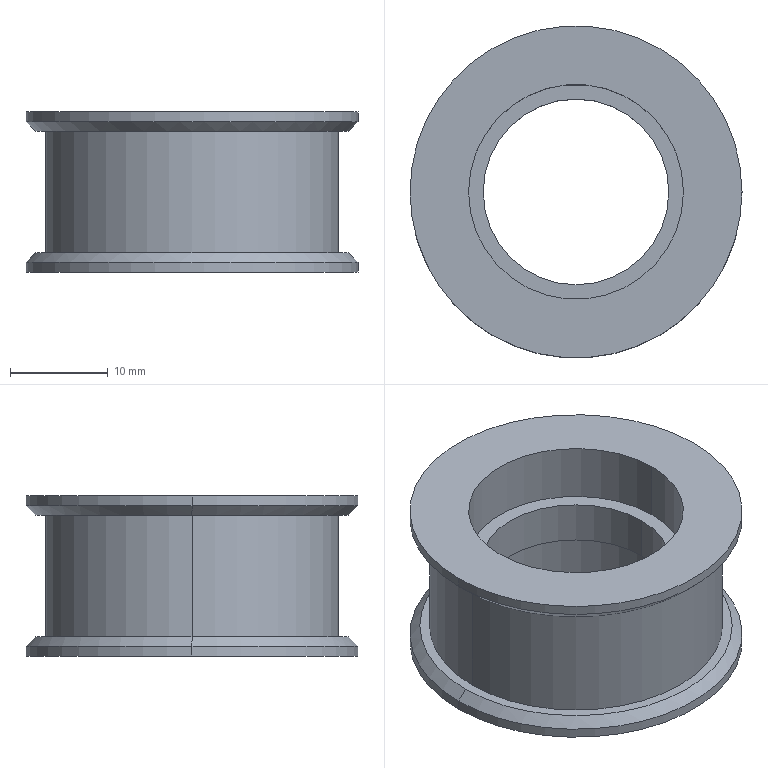Part | STEP file | PN_0033 Mount electronic clip wheel connector | 1 solid | 22 faces | box 34 x 34 x 16.4 mm | volume 6483 mm3 | cylinder 12 | plane 6 | cone 4 | commonest cylinder face diameters 22 x4 34 x4 19 x2 30 x2
STEP:
#1=CARTESIAN_POINT('',(0.,0.,0.));
#2=DIRECTION('',(0.,0.,1.));
#3=DIRECTION('',(1.,0.,0.));
#4=AXIS2_PLACEMENT_3D('',#1,#2,#3);
#5=CARTESIAN_POINT('',(16.,0.,0.));
#6=VERTEX_POINT('',#5);
#7=CARTESIAN_POINT('',(-16.,0.,0.));
#8=VERTEX_POINT('',#7);
#9=CARTESIAN_POINT('',(0.,0.,0.));
#10=DIRECTION('',(0.,0.,1.));
#11=DIRECTION('',(-1.,0.,0.));
#12=AXIS2_PLACEMENT_3D('',#9,#10,#11);
#13=CIRCLE('',#12,16.);
#14=CARTESIAN_POINT('',(0.,0.,-1.));
#15=DIRECTION('',(0.,0.,-1.));
#16=DIRECTION('',(-1.,0.,0.));
#17=AXIS2_PLACEMENT_3D('',#14,#15,#16);
#18=CONICAL_SURFACE('',#17,17.,0.7854);
#19=CARTESIAN_POINT('',(6.283,-1.));
#20=DIRECTION('',(-1.,0.));
#21=VECTOR('',#20,1.);
#22=LINE('',#19,#21);
#23=(GEOMETRIC_REPRESENTATION_CONTEXT(2)PARAMETRIC_REPRESENTATION_CONTEXT()REPRESENTATION_CONTEXT('',''));
#24=DEFINITIONAL_REPRESENTATION('',(#22),#23);
#25=PCURVE('',#18,#24);
#26=CARTESIAN_POINT('',(0.,0.,0.));
#27=DIRECTION('',(0.,0.,-1.));
#28=DIRECTION('',(-1.,0.,0.));
#29=AXIS2_PLACEMENT_3D('',#26,#27,#28);
#30=PLANE('',#29);
#31=CARTESIAN_POINT('',(16.,0.));
#32=CARTESIAN_POINT('',(16.,-27.713));
#33=CARTESIAN_POINT('',(-8.,-13.856));
#34=CARTESIAN_POINT('',(-32.,0.));
#35=CARTESIAN_POINT('',(-8.,13.856));
#36=CARTESIAN_POINT('',(16.,27.713));
#37=CARTESIAN_POINT('',(16.,0.));
#38=(BOUNDED_CURVE()B_SPLINE_CURVE(2,(#31,#32,#33,#34,#35,#36,#37),.UNSPECIFIED.,.T.,.F.)B_SPLINE_CURVE_WITH_KNOTS((1,2,2,2,2,1),(-2.094,0.,2.094,4.189,6.283,8.378),.UNSPECIFIED.)CURVE()GEOMETRIC_REPRESENTATION_ITEM()RATIONAL_B_SPLINE_CURVE((1.,0.5,1.,0.5,1.,0.5,1.))REPRESENTATION_ITEM(''));
#39=(GEOMETRIC_REPRESENTATION_CONTEXT(2)PARAMETRIC_REPRESENTATION_CONTEXT()REPRESENTATION_CONTEXT('',''));
#40=DEFINITIONAL_REPRESENTATION('',(#38),#39);
#41=PCURVE('',#30,#40);
#42=SURFACE_CURVE('',#13,(#25,#41),.PCURVE_S1.);
#43=EDGE_CURVE('',#6,#8,#42,.T.);
#44=ORIENTED_EDGE('',*,*,#43,.F.);
#45=CARTESIAN_POINT('',(17.,0.,-1.));
#46=VERTEX_POINT('',#45);
#47=CARTESIAN_POINT('',(17.,0.,-1.));
#48=DIRECTION('',(0.7071,0.,-0.7071));
#49=VECTOR('',#48,1.);
#50=LINE('',#47,#49);
#51=CARTESIAN_POINT('',(3.142,0.));
#52=DIRECTION('',(0.,1.));
#53=VECTOR('',#52,1.);
#54=LINE('',#51,#53);
#55=(GEOMETRIC_REPRESENTATION_CONTEXT(2)PARAMETRIC_REPRESENTATION_CONTEXT()REPRESENTATION_CONTEXT('',''));
#56=DEFINITIONAL_REPRESENTATION('',(#54),#55);
#57=PCURVE('',#18,#56);
#58=CARTESIAN_POINT('',(0.,0.,-1.));
#59=DIRECTION('',(0.,0.,-1.));
#60=DIRECTION('',(-1.,0.,0.));
#61=AXIS2_PLACEMENT_3D('',#58,#59,#60);
#62=CONICAL_SURFACE('',#61,17.,0.7854);
#63=CARTESIAN_POINT('',(3.142,0.));
#64=DIRECTION('',(0.,1.));
#65=VECTOR('',#64,1.);
#66=LINE('',#63,#65);
#67=(GEOMETRIC_REPRESENTATION_CONTEXT(2)PARAMETRIC_REPRESENTATION_CONTEXT()REPRESENTATION_CONTEXT('',''));
#68=DEFINITIONAL_REPRESENTATION('',(#66),#67);
#69=PCURVE('',#62,#68);
#70=SURFACE_CURVE('',#50,(#57,#69),.PCURVE_S1.);
#71=EDGE_CURVE('',#6,#46,#70,.T.);
#72=ORIENTED_EDGE('',*,*,#71,.T.);
#73=CARTESIAN_POINT('',(-17.,0.,-1.));
#74=VERTEX_POINT('',#73);
#75=CARTESIAN_POINT('',(0.,0.,-1.));
#76=DIRECTION('',(0.,0.,-1.));
#77=DIRECTION('',(-1.,0.,0.));
#78=AXIS2_PLACEMENT_3D('',#75,#76,#77);
#79=CIRCLE('',#78,17.);
#80=CARTESIAN_POINT('',(0.,0.));
#81=DIRECTION('',(1.,0.));
#82=VECTOR('',#81,1.);
#83=LINE('',#80,#82);
#84=(GEOMETRIC_REPRESENTATION_CONTEXT(2)PARAMETRIC_REPRESENTATION_CONTEXT()REPRESENTATION_CONTEXT('',''));
#85=DEFINITIONAL_REPRESENTATION('',(#83),#84);
#86=PCURVE('',#18,#85);
#87=CARTESIAN_POINT('',(0.,0.,-2.));
#88=DIRECTION('',(0.,0.,1.));
#89=DIRECTION('',(1.,0.,0.));
#90=AXIS2_PLACEMENT_3D('',#87,#88,#89);
#91=CYLINDRICAL_SURFACE('',#90,17.);
#92=CARTESIAN_POINT('',(3.142,1.));
#93=DIRECTION('',(-1.,0.));
#94=VECTOR('',#93,1.);
#95=LINE('',#92,#94);
#96=(GEOMETRIC_REPRESENTATION_CONTEXT(2)PARAMETRIC_REPRESENTATION_CONTEXT()REPRESENTATION_CONTEXT('',''));
#97=DEFINITIONAL_REPRESENTATION('',(#95),#96);
#98=PCURVE('',#91,#97);
#99=SURFACE_CURVE('',#79,(#86,#98),.PCURVE_S1.);
#100=EDGE_CURVE('',#74,#46,#99,.T.);
#101=ORIENTED_EDGE('',*,*,#100,.F.);
#102=CARTESIAN_POINT('',(-17.,0.,-1.));
#103=DIRECTION('',(-0.7071,0.,-0.7071));
#104=VECTOR('',#103,1.);
#105=LINE('',#102,#104);
#106=CARTESIAN_POINT('',(0.,0.));
#107=DIRECTION('',(0.,1.));
#108=VECTOR('',#107,1.);
#109=LINE('',#106,#108);
#110=(GEOMETRIC_REPRESENTATION_CONTEXT(2)PARAMETRIC_REPRESENTATION_CONTEXT()REPRESENTATION_CONTEXT('',''));
#111=DEFINITIONAL_REPRESENTATION('',(#109),#110);
#112=PCURVE('',#18,#111);
#113=CARTESIAN_POINT('',(6.283,0.));
#114=DIRECTION('',(0.,1.));
#115=VECTOR('',#114,1.);
#116=LINE('',#113,#115);
#117=(GEOMETRIC_REPRESENTATION_CONTEXT(2)PARAMETRIC_REPRESENTATION_CONTEXT()REPRESENTATION_CONTEXT('',''));
#118=DEFINITIONAL_REPRESENTATION('',(#116),#117);
#119=PCURVE('',#62,#118);
#120=SURFACE_CURVE('',#105,(#112,#119),.PCURVE_S1.);
#121=EDGE_CURVE('',#8,#74,#120,.T.);
#122=ORIENTED_EDGE('',*,*,#121,.F.);
#123=EDGE_LOOP('',(#44,#72,#101,#122));
#124=FACE_BOUND('',#123,.T.);
#125=ADVANCED_FACE('',(#124),#18,.T.);
#126=CARTESIAN_POINT('',(-16.,0.,12.4));
#127=VERTEX_POINT('',#126);
#128=CARTESIAN_POINT('',(16.,0.,12.4));
#129=VERTEX_POINT('',#128);
#130=CARTESIAN_POINT('',(0.,0.,12.4));
#131=DIRECTION('',(0.,0.,-1.));
#132=DIRECTION('',(1.,0.,0.));
#133=AXIS2_PLACEMENT_3D('',#130,#131,#132);
#134=CIRCLE('',#133,16.);
#135=CARTESIAN_POINT('',(0.,0.,13.4));
#136=DIRECTION('',(0.,0.,1.));
#137=DIRECTION('',(1.,0.,0.));
#138=AXIS2_PLACEMENT_3D('',#135,#136,#137);
#139=CONICAL_SURFACE('',#138,17.,0.7854);
#140=CARTESIAN_POINT('',(6.283,-1.));
#141=DIRECTION('',(-1.,0.));
#142=VECTOR('',#141,1.);
#143=LINE('',#140,#142);
#144=(GEOMETRIC_REPRESENTATION_CONTEXT(2)PARAMETRIC_REPRESENTATION_CONTEXT()REPRESENTATION_CONTEXT('',''));
#145=DEFINITIONAL_REPRESENTATION('',(#143),#144);
#146=PCURVE('',#139,#145);
#147=CARTESIAN_POINT('',(0.,0.,12.4));
#148=DIRECTION('',(0.,0.,1.));
#149=DIRECTION('',(1.,0.,0.));
#150=AXIS2_PLACEMENT_3D('',#147,#148,#149);
#151=PLANE('',#150);
#152=CARTESIAN_POINT('',(16.,0.));
#153=CARTESIAN_POINT('',(16.,-27.713));
#154=CARTESIAN_POINT('',(-8.,-13.856));
#155=CARTESIAN_POINT('',(-32.,0.));
#156=CARTESIAN_POINT('',(-8.,13.856));
#157=CARTESIAN_POINT('',(16.,27.713));
#158=CARTESIAN_POINT('',(16.,0.));
#159=(BOUNDED_CURVE()B_SPLINE_CURVE(2,(#152,#153,#154,#155,#156,#157,#158),.UNSPECIFIED.,.T.,.F.)B_SPLINE_CURVE_WITH_KNOTS((1,2,2,2,2,1),(-2.094,0.,2.094,4.189,6.283,8.378),.UNSPECIFIED.)CURVE()GEOMETRIC_REPRESENTATION_ITEM()RATIONAL_B_SPLINE_CURVE((1.,0.5,1.,0.5,1.,0.5,1.))REPRESENTATION_ITEM(''));
#160=(GEOMETRIC_REPRESENTATION_CONTEXT(2)PARAMETRIC_REPRESENTATION_CONTEXT()REPRESENTATION_CONTEXT('',''));
#161=DEFINITIONAL_REPRESENTATION('',(#159),#160);
#162=PCURVE('',#151,#161);
#163=SURFACE_CURVE('',#134,(#146,#162),.PCURVE_S1.);
#164=EDGE_CURVE('',#127,#129,#163,.T.);
#165=ORIENTED_EDGE('',*,*,#164,.F.);
#166=CARTESIAN_POINT('',(-17.,0.,13.4));
#167=VERTEX_POINT('',#166);
#168=CARTESIAN_POINT('',(-17.,0.,13.4));
#169=DIRECTION('',(-0.7071,0.,0.7071));
#170=VECTOR('',#169,1.);
#171=LINE('',#168,#170);
#172=CARTESIAN_POINT('',(3.142,0.));
#173=DIRECTION('',(0.,1.));
#174=VECTOR('',#173,1.);
#175=LINE('',#172,#174);
#176=(GEOMETRIC_REPRESENTATION_CONTEXT(2)PARAMETRIC_REPRESENTATION_CONTEXT()REPRESENTATION_CONTEXT('',''));
#177=DEFINITIONAL_REPRESENTATION('',(#175),#176);
#178=PCURVE('',#139,#177);
#179=CARTESIAN_POINT('',(0.,0.,13.4));
#180=DIRECTION('',(0.,0.,1.));
#181=DIRECTION('',(1.,0.,0.));
#182=AXIS2_PLACEMENT_3D('',#179,#180,#181);
#183=CONICAL_SURFACE('',#182,17.,0.7854);
#184=CARTESIAN_POINT('',(3.142,0.));
#185=DIRECTION('',(0.,1.));
#186=VECTOR('',#185,1.);
#187=LINE('',#184,#186);
#188=(GEOMETRIC_REPRESENTATION_CONTEXT(2)PARAMETRIC_REPRESENTATION_CONTEXT()REPRESENTATION_CONTEXT('',''));
#189=DEFINITIONAL_REPRESENTATION('',(#187),#188);
#190=PCURVE('',#183,#189);
#191=SURFACE_CURVE('',#171,(#178,#190),.PCURVE_S1.);
#192=EDGE_CURVE('',#127,#167,#191,.T.);
#193=ORIENTED_EDGE('',*,*,#192,.T.);
#194=CARTESIAN_POINT('',(17.,0.,13.4));
#195=VERTEX_POINT('',#194);
#196=CARTESIAN_POINT('',(0.,0.,13.4));
#197=DIRECTION('',(0.,0.,1.));
#198=DIRECTION('',(1.,0.,0.));
#199=AXIS2_PLACEMENT_3D('',#196,#197,#198);
#200=CIRCLE('',#199,17.);
#201=CARTESIAN_POINT('',(0.,0.));
#202=DIRECTION('',(1.,0.));
#203=VECTOR('',#202,1.);
#204=LINE('',#201,#203);
#205=(GEOMETRIC_REPRESENTATION_CONTEXT(2)PARAMETRIC_REPRESENTATION_CONTEXT()REPRESENTATION_CONTEXT('',''));
#206=DEFINITIONAL_REPRESENTATION('',(#204),#205);
#207=PCURVE('',#139,#206);
#208=CARTESIAN_POINT('',(0.,0.,14.4));
#209=DIRECTION('',(0.,0.,-1.));
#210=DIRECTION('',(-1.,0.,0.));
#211=AXIS2_PLACEMENT_3D('',#208,#209,#210);
#212=CYLINDRICAL_SURFACE('',#211,17.);
#213=CARTESIAN_POINT('',(3.142,1.));
#214=DIRECTION('',(-1.,0.));
#215=VECTOR('',#214,1.);
#216=LINE('',#213,#215);
#217=(GEOMETRIC_REPRESENTATION_CONTEXT(2)PARAMETRIC_REPRESENTATION_CONTEXT()REPRESENTATION_CONTEXT('',''));
#218=DEFINITIONAL_REPRESENTATION('',(#216),#217);
#219=PCURVE('',#212,#218);
#220=SURFACE_CURVE('',#200,(#207,#219),.PCURVE_S1.);
#221=EDGE_CURVE('',#195,#167,#220,.T.);
#222=ORIENTED_EDGE('',*,*,#221,.F.);
#223=CARTESIAN_POINT('',(17.,0.,13.4));
#224=DIRECTION('',(0.7071,0.,0.7071));
#225=VECTOR('',#224,1.);
#226=LINE('',#223,#225);
#227=CARTESIAN_POINT('',(0.,0.));
#228=DIRECTION('',(0.,1.));
#229=VECTOR('',#228,1.);
#230=LINE('',#227,#229);
#231=(GEOMETRIC_REPRESENTATION_CONTEXT(2)PARAMETRIC_REPRESENTATION_CONTEXT()REPRESENTATION_CONTEXT('',''));
#232=DEFINITIONAL_REPRESENTATION('',(#230),#231);
#233=PCURVE('',#139,#232);
#234=CARTESIAN_POINT('',(6.283,0.));
#235=DIRECTION('',(0.,1.));
#236=VECTOR('',#235,1.);
#237=LINE('',#234,#236);
#238=(GEOMETRIC_REPRESENTATION_CONTEXT(2)PARAMETRIC_REPRESENTATION_CONTEXT()REPRESENTATION_CONTEXT('',''));
#239=DEFINITIONAL_REPRESENTATION('',(#237),#238);
#240=PCURVE('',#183,#239);
#241=SURFACE_CURVE('',#226,(#233,#240),.PCURVE_S1.);
#242=EDGE_CURVE('',#129,#195,#241,.T.);
#243=ORIENTED_EDGE('',*,*,#242,.F.);
#244=EDGE_LOOP('',(#165,#193,#222,#243));
#245=FACE_BOUND('',#244,.T.);
#246=ADVANCED_FACE('',(#245),#139,.T.);
#247=CARTESIAN_POINT('',(-11.,0.,4.));
#248=VERTEX_POINT('',#247);
#249=CARTESIAN_POINT('',(-11.,0.,-2.));
#250=VERTEX_POINT('',#249);
#251=CARTESIAN_POINT('',(-11.,0.,4.));
#252=DIRECTION('',(0.,0.,-1.));
#253=VECTOR('',#252,1.);
#254=LINE('',#251,#253);
#255=CARTESIAN_POINT('',(0.,0.,4.));
#256=DIRECTION('',(0.,0.,-1.));
#257=DIRECTION('',(-1.,0.,0.));
#258=AXIS2_PLACEMENT_3D('',#255,#256,#257);
#259=CYLINDRICAL_SURFACE('',#258,11.);
#260=CARTESIAN_POINT('',(6.283,0.));
#261=DIRECTION('',(0.,1.));
#262=VECTOR('',#261,1.);
#263=LINE('',#260,#262);
#264=(GEOMETRIC_REPRESENTATION_CONTEXT(2)PARAMETRIC_REPRESENTATION_CONTEXT()REPRESENTATION_CONTEXT('',''));
#265=DEFINITIONAL_REPRESENTATION('',(#263),#264);
#266=PCURVE('',#259,#265);
#267=CARTESIAN_POINT('',(0.,0.,4.));
#268=DIRECTION('',(0.,0.,-1.));
#269=DIRECTION('',(-1.,0.,0.));
#270=AXIS2_PLACEMENT_3D('',#267,#268,#269);
#271=CYLINDRICAL_SURFACE('',#270,11.);
#272=CARTESIAN_POINT('',(0.,0.));
#273=DIRECTION('',(0.,1.));
#274=VECTOR('',#273,1.);
#275=LINE('',#272,#274);
#276=(GEOMETRIC_REPRESENTATION_CONTEXT(2)PARAMETRIC_REPRESENTATION_CONTEXT()REPRESENTATION_CONTEXT('',''));
#277=DEFINITIONAL_REPRESENTATION('',(#275),#276);
#278=PCURVE('',#271,#277);
#279=SURFACE_CURVE('',#254,(#266,#278),.PCURVE_S1.);
#280=EDGE_CURVE('',#248,#250,#279,.T.);
#281=ORIENTED_EDGE('',*,*,#280,.T.);
#282=CARTESIAN_POINT('',(11.,0.,-2.));
#283=VERTEX_POINT('',#282);
#284=CARTESIAN_POINT('',(0.,0.,-2.));
#285=DIRECTION('',(0.,0.,-1.));
#286=DIRECTION('',(-1.,0.,0.));
#287=AXIS2_PLACEMENT_3D('',#284,#285,#286);
#288=CIRCLE('',#287,11.);
#289=CARTESIAN_POINT('',(0.,6.));
#290=DIRECTION('',(1.,0.));
#291=VECTOR('',#290,1.);
#292=LINE('',#289,#291);
#293=(GEOMETRIC_REPRESENTATION_CONTEXT(2)PARAMETRIC_REPRESENTATION_CONTEXT()REPRESENTATION_CONTEXT('',''));
#294=DEFINITIONAL_REPRESENTATION('',(#292),#293);
#295=PCURVE('',#259,#294);
#296=CARTESIAN_POINT('',(0.,0.,-2.));
#297=DIRECTION('',(0.,0.,-1.));
#298=DIRECTION('',(-1.,0.,0.));
#299=AXIS2_PLACEMENT_3D('',#296,#297,#298);
#300=PLANE('',#299);
#301=CARTESIAN_POINT('',(0.,0.));
#302=DIRECTION('',(1.,0.));
#303=AXIS2_PLACEMENT_2D('',#301,#302);
#304=CIRCLE('',#303,11.);
#305=(GEOMETRIC_REPRESENTATION_CONTEXT(2)PARAMETRIC_REPRESENTATION_CONTEXT()REPRESENTATION_CONTEXT('',''));
#306=DEFINITIONAL_REPRESENTATION('',(#304),#305);
#307=PCURVE('',#300,#306);
#308=SURFACE_CURVE('',#288,(#295,#307),.PCURVE_S1.);
#309=EDGE_CURVE('',#283,#250,#308,.T.);
#310=ORIENTED_EDGE('',*,*,#309,.F.);
#311=CARTESIAN_POINT('',(11.,0.,4.));
#312=VERTEX_POINT('',#311);
#313=CARTESIAN_POINT('',(11.,0.,4.));
#314=DIRECTION('',(0.,0.,-1.));
#315=VECTOR('',#314,1.);
#316=LINE('',#313,#315);
#317=CARTESIAN_POINT('',(3.142,0.));
#318=DIRECTION('',(0.,1.));
#319=VECTOR('',#318,1.);
#320=LINE('',#317,#319);
#321=(GEOMETRIC_REPRESENTATION_CONTEXT(2)PARAMETRIC_REPRESENTATION_CONTEXT()REPRESENTATION_CONTEXT('',''));
#322=DEFINITIONAL_REPRESENTATION('',(#320),#321);
#323=PCURVE('',#259,#322);
#324=CARTESIAN_POINT('',(3.142,0.));
#325=DIRECTION('',(0.,1.));
#326=VECTOR('',#325,1.);
#327=LINE('',#324,#326);
#328=(GEOMETRIC_REPRESENTATION_CONTEXT(2)PARAMETRIC_REPRESENTATION_CONTEXT()REPRESENTATION_CONTEXT('',''));
#329=DEFINITIONAL_REPRESENTATION('',(#327),#328);
#330=PCURVE('',#271,#329);
#331=SURFACE_CURVE('',#316,(#323,#330),.PCURVE_S1.);
#332=EDGE_CURVE('',#312,#283,#331,.T.);
#333=ORIENTED_EDGE('',*,*,#332,.F.);
#334=CARTESIAN_POINT('',(0.,0.,4.));
#335=DIRECTION('',(0.,0.,-1.));
#336=DIRECTION('',(-1.,0.,0.));
#337=AXIS2_PLACEMENT_3D('',#334,#335,#336);
#338=CIRCLE('',#337,11.);
#339=CARTESIAN_POINT('',(0.,0.));
#340=DIRECTION('',(1.,0.));
#341=VECTOR('',#340,1.);
#342=LINE('',#339,#341);
#343=(GEOMETRIC_REPRESENTATION_CONTEXT(2)PARAMETRIC_REPRESENTATION_CONTEXT()REPRESENTATION_CONTEXT('',''));
#344=DEFINITIONAL_REPRESENTATION('',(#342),#343);
#345=PCURVE('',#259,#344);
#346=CARTESIAN_POINT('',(0.,0.,4.));
#347=DIRECTION('',(0.,0.,-1.));
#348=DIRECTION('',(-1.,0.,0.));
#349=AXIS2_PLACEMENT_3D('',#346,#347,#348);
#350=PLANE('',#349);
#351=CARTESIAN_POINT('',(0.,0.));
#352=DIRECTION('',(1.,0.));
#353=AXIS2_PLACEMENT_2D('',#351,#352);
#354=CIRCLE('',#353,11.);
#355=(GEOMETRIC_REPRESENTATION_CONTEXT(2)PARAMETRIC_REPRESENTATION_CONTEXT()REPRESENTATION_CONTEXT('',''));
#356=DEFINITIONAL_REPRESENTATION('',(#354),#355);
#357=PCURVE('',#350,#356);
#358=SURFACE_CURVE('',#338,(#345,#357),.PCURVE_S1.);
#359=EDGE_CURVE('',#312,#248,#358,.T.);
#360=ORIENTED_EDGE('',*,*,#359,.T.);
#361=EDGE_LOOP('',(#281,#310,#333,#360));
#362=FACE_BOUND('',#361,.F.);
#363=ADVANCED_FACE('',(#362),#259,.F.);
#364=CARTESIAN_POINT('',(11.,0.,8.4));
#365=VERTEX_POINT('',#364);
#366=CARTESIAN_POINT('',(11.,0.,14.4));
#367=VERTEX_POINT('',#366);
#368=CARTESIAN_POINT('',(11.,0.,8.4));
#369=DIRECTION('',(0.,0.,1.));
#370=VECTOR('',#369,1.);
#371=LINE('',#368,#370);
#372=CARTESIAN_POINT('',(0.,0.,8.4));
#373=DIRECTION('',(0.,0.,1.));
#374=DIRECTION('',(1.,0.,0.));
#375=AXIS2_PLACEMENT_3D('',#372,#373,#374);
#376=CYLINDRICAL_SURFACE('',#375,11.);
#377=CARTESIAN_POINT('',(6.283,0.));
#378=DIRECTION('',(0.,1.));
#379=VECTOR('',#378,1.);
#380=LINE('',#377,#379);
#381=(GEOMETRIC_REPRESENTATION_CONTEXT(2)PARAMETRIC_REPRESENTATION_CONTEXT()REPRESENTATION_CONTEXT('',''));
#382=DEFINITIONAL_REPRESENTATION('',(#380),#381);
#383=PCURVE('',#376,#382);
#384=CARTESIAN_POINT('',(0.,0.,8.4));
#385=DIRECTION('',(0.,0.,1.));
#386=DIRECTION('',(1.,0.,0.));
#387=AXIS2_PLACEMENT_3D('',#384,#385,#386);
#388=CYLINDRICAL_SURFACE('',#387,11.);
#389=CARTESIAN_POINT('',(0.,0.));
#390=DIRECTION('',(0.,1.));
#391=VECTOR('',#390,1.);
#392=LINE('',#389,#391);
#393=(GEOMETRIC_REPRESENTATION_CONTEXT(2)PARAMETRIC_REPRESENTATION_CONTEXT()REPRESENTATION_CONTEXT('',''));
#394=DEFINITIONAL_REPRESENTATION('',(#392),#393);
#395=PCURVE('',#388,#394);
#396=SURFACE_CURVE('',#371,(#383,#395),.PCURVE_S1.);
#397=EDGE_CURVE('',#365,#367,#396,.T.);
#398=ORIENTED_EDGE('',*,*,#397,.T.);
#399=CARTESIAN_POINT('',(-11.,0.,14.4));
#400=VERTEX_POINT('',#399);
#401=CARTESIAN_POINT('',(0.,0.,14.4));
#402=DIRECTION('',(0.,0.,1.));
#403=DIRECTION('',(1.,0.,0.));
#404=AXIS2_PLACEMENT_3D('',#401,#402,#403);
#405=CIRCLE('',#404,11.);
#406=CARTESIAN_POINT('',(0.,6.));
#407=DIRECTION('',(1.,0.));
#408=VECTOR('',#407,1.);
#409=LINE('',#406,#408);
#410=(GEOMETRIC_REPRESENTATION_CONTEXT(2)PARAMETRIC_REPRESENTATION_CONTEXT()REPRESENTATION_CONTEXT('',''));
#411=DEFINITIONAL_REPRESENTATION('',(#409),#410);
#412=PCURVE('',#376,#411);
#413=CARTESIAN_POINT('',(0.,0.,14.4));
#414=DIRECTION('',(0.,0.,1.));
#415=DIRECTION('',(1.,0.,0.));
#416=AXIS2_PLACEMENT_3D('',#413,#414,#415);
#417=PLANE('',#416);
#418=CARTESIAN_POINT('',(0.,0.));
#419=DIRECTION('',(1.,0.));
#420=AXIS2_PLACEMENT_2D('',#418,#419);
#421=CIRCLE('',#420,11.);
#422=(GEOMETRIC_REPRESENTATION_CONTEXT(2)PARAMETRIC_REPRESENTATION_CONTEXT()REPRESENTATION_CONTEXT('',''));
#423=DEFINITIONAL_REPRESENTATION('',(#421),#422);
#424=PCURVE('',#417,#423);
#425=SURFACE_CURVE('',#405,(#412,#424),.PCURVE_S1.);
#426=EDGE_CURVE('',#400,#367,#425,.T.);
#427=ORIENTED_EDGE('',*,*,#426,.F.);
#428=CARTESIAN_POINT('',(-11.,0.,8.4));
#429=VERTEX_POINT('',#428);
#430=CARTESIAN_POINT('',(-11.,0.,8.4));
#431=DIRECTION('',(0.,0.,1.));
#432=VECTOR('',#431,1.);
#433=LINE('',#430,#432);
#434=CARTESIAN_POINT('',(3.142,0.));
#435=DIRECTION('',(0.,1.));
#436=VECTOR('',#435,1.);
#437=LINE('',#434,#436);
#438=(GEOMETRIC_REPRESENTATION_CONTEXT(2)PARAMETRIC_REPRESENTATION_CONTEXT()REPRESENTATION_CONTEXT('',''));
#439=DEFINITIONAL_REPRESENTATION('',(#437),#438);
#440=PCURVE('',#376,#439);
#441=CARTESIAN_POINT('',(3.142,0.));
#442=DIRECTION('',(0.,1.));
#443=VECTOR('',#442,1.);
#444=LINE('',#441,#443);
#445=(GEOMETRIC_REPRESENTATION_CONTEXT(2)PARAMETRIC_REPRESENTATION_CONTEXT()REPRESENTATION_CONTEXT('',''));
#446=DEFINITIONAL_REPRESENTATION('',(#444),#445);
#447=PCURVE('',#388,#446);
#448=SURFACE_CURVE('',#433,(#440,#447),.PCURVE_S1.);
#449=EDGE_CURVE('',#429,#400,#448,.T.);
#450=ORIENTED_EDGE('',*,*,#449,.F.);
#451=CARTESIAN_POINT('',(0.,0.,8.4));
#452=DIRECTION('',(0.,0.,1.));
#453=DIRECTION('',(1.,0.,0.));
#454=AXIS2_PLACEMENT_3D('',#451,#452,#453);
#455=CIRCLE('',#454,11.);
#456=CARTESIAN_POINT('',(0.,0.));
#457=DIRECTION('',(1.,0.));
#458=VECTOR('',#457,1.);
#459=LINE('',#456,#458);
#460=(GEOMETRIC_REPRESENTATION_CONTEXT(2)PARAMETRIC_REPRESENTATION_CONTEXT()REPRESENTATION_CONTEXT('',''));
#461=DEFINITIONAL_REPRESENTATION('',(#459),#460);
#462=PCURVE('',#376,#461);
#463=CARTESIAN_POINT('',(0.,0.,8.4));
#464=DIRECTION('',(0.,0.,1.));
#465=DIRECTION('',(1.,0.,0.));
#466=AXIS2_PLACEMENT_3D('',#463,#464,#465);
#467=PLANE('',#466);
#468=CARTESIAN_POINT('',(0.,0.));
#469=DIRECTION('',(1.,0.));
#470=AXIS2_PLACEMENT_2D('',#468,#469);
#471=CIRCLE('',#470,11.);
#472=(GEOMETRIC_REPRESENTATION_CONTEXT(2)PARAMETRIC_REPRESENTATION_CONTEXT()REPRESENTATION_CONTEXT('',''));
#473=DEFINITIONAL_REPRESENTATION('',(#471),#472);
#474=PCURVE('',#467,#473);
#475=SURFACE_CURVE('',#455,(#462,#474),.PCURVE_S1.);
#476=EDGE_CURVE('',#429,#365,#475,.T.);
#477=ORIENTED_EDGE('',*,*,#476,.T.);
#478=EDGE_LOOP('',(#398,#427,#450,#477));
#479=FACE_BOUND('',#478,.F.);
#480=ADVANCED_FACE('',(#479),#376,.F.);
#481=CARTESIAN_POINT('',(-17.,0.,-2.));
#482=VERTEX_POINT('',#481);
#483=CARTESIAN_POINT('',(17.,0.,-2.));
#484=VERTEX_POINT('',#483);
#485=CARTESIAN_POINT('',(0.,0.,-2.));
#486=DIRECTION('',(0.,0.,-1.));
#487=DIRECTION('',(-1.,0.,0.));
#488=AXIS2_PLACEMENT_3D('',#485,#486,#487);
#489=CIRCLE('',#488,17.);
#490=CARTESIAN_POINT('',(3.142,0.));
#491=DIRECTION('',(-1.,0.));
#492=VECTOR('',#491,1.);
#493=LINE('',#490,#492);
#494=(GEOMETRIC_REPRESENTATION_CONTEXT(2)PARAMETRIC_REPRESENTATION_CONTEXT()REPRESENTATION_CONTEXT('',''));
#495=DEFINITIONAL_REPRESENTATION('',(#493),#494);
#496=PCURVE('',#91,#495);
#497=CARTESIAN_POINT('',(0.,0.));
#498=DIRECTION('',(1.,0.));
#499=AXIS2_PLACEMENT_2D('',#497,#498);
#500=CIRCLE('',#499,17.);
#501=(GEOMETRIC_REPRESENTATION_CONTEXT(2)PARAMETRIC_REPRESENTATION_CONTEXT()REPRESENTATION_CONTEXT('',''));
#502=DEFINITIONAL_REPRESENTATION('',(#500),#501);
#503=PCURVE('',#300,#502);
#504=SURFACE_CURVE('',#489,(#496,#503),.PCURVE_S1.);
#505=EDGE_CURVE('',#482,#484,#504,.T.);
#506=ORIENTED_EDGE('',*,*,#505,.F.);
#507=CARTESIAN_POINT('',(-17.,0.,-2.));
#508=DIRECTION('',(0.,0.,1.));
#509=VECTOR('',#508,1.);
#510=LINE('',#507,#509);
#511=CARTESIAN_POINT('',(3.142,0.));
#512=DIRECTION('',(0.,1.));
#513=VECTOR('',#512,1.);
#514=LINE('',#511,#513);
#515=(GEOMETRIC_REPRESENTATION_CONTEXT(2)PARAMETRIC_REPRESENTATION_CONTEXT()REPRESENTATION_CONTEXT('',''));
#516=DEFINITIONAL_REPRESENTATION('',(#514),#515);
#517=PCURVE('',#91,#516);
#518=CARTESIAN_POINT('',(0.,0.,-2.));
#519=DIRECTION('',(0.,0.,1.));
#520=DIRECTION('',(1.,0.,0.));
#521=AXIS2_PLACEMENT_3D('',#518,#519,#520);
#522=CYLINDRICAL_SURFACE('',#521,17.);
#523=CARTESIAN_POINT('',(3.142,0.));
#524=DIRECTION('',(0.,1.));
#525=VECTOR('',#524,1.);
#526=LINE('',#523,#525);
#527=(GEOMETRIC_REPRESENTATION_CONTEXT(2)PARAMETRIC_REPRESENTATION_CONTEXT()REPRESENTATION_CONTEXT('',''));
#528=DEFINITIONAL_REPRESENTATION('',(#526),#527);
#529=PCURVE('',#522,#528);
#530=SURFACE_CURVE('',#510,(#517,#529),.PCURVE_S1.);
#531=EDGE_CURVE('',#482,#74,#530,.T.);
#532=ORIENTED_EDGE('',*,*,#531,.T.);
#533=ORIENTED_EDGE('',*,*,#100,.T.);
#534=CARTESIAN_POINT('',(17.,0.,-2.));
#535=DIRECTION('',(0.,0.,1.));
#536=VECTOR('',#535,1.);
#537=LINE('',#534,#536);
#538=CARTESIAN_POINT('',(0.,0.));
#539=DIRECTION('',(0.,1.));
#540=VECTOR('',#539,1.);
#541=LINE('',#538,#540);
#542=(GEOMETRIC_REPRESENTATION_CONTEXT(2)PARAMETRIC_REPRESENTATION_CONTEXT()REPRESENTATION_CONTEXT('',''));
#543=DEFINITIONAL_REPRESENTATION('',(#541),#542);
#544=PCURVE('',#91,#543);
#545=CARTESIAN_POINT('',(6.283,0.));
#546=DIRECTION('',(0.,1.));
#547=VECTOR('',#546,1.);
#548=LINE('',#545,#547);
#549=(GEOMETRIC_REPRESENTATION_CONTEXT(2)PARAMETRIC_REPRESENTATION_CONTEXT()REPRESENTATION_CONTEXT('',''));
#550=DEFINITIONAL_REPRESENTATION('',(#548),#549);
#551=PCURVE('',#522,#550);
#552=SURFACE_CURVE('',#537,(#544,#551),.PCURVE_S1.);
#553=EDGE_CURVE('',#484,#46,#552,.T.);
#554=ORIENTED_EDGE('',*,*,#553,.F.);
#555=EDGE_LOOP('',(#506,#532,#533,#554));
#556=FACE_BOUND('',#555,.T.);
#557=ADVANCED_FACE('',(#556),#91,.T.);
#558=CARTESIAN_POINT('',(17.,0.,14.4));
#559=VERTEX_POINT('',#558);
#560=CARTESIAN_POINT('',(-17.,0.,14.4));
#561=VERTEX_POINT('',#560);
#562=CARTESIAN_POINT('',(0.,0.,14.4));
#563=DIRECTION('',(0.,0.,1.));
#564=DIRECTION('',(1.,0.,0.));
#565=AXIS2_PLACEMENT_3D('',#562,#563,#564);
#566=CIRCLE('',#565,17.);
#567=CARTESIAN_POINT('',(3.142,0.));
#568=DIRECTION('',(-1.,0.));
#569=VECTOR('',#568,1.);
#570=LINE('',#567,#569);
#571=(GEOMETRIC_REPRESENTATION_CONTEXT(2)PARAMETRIC_REPRESENTATION_CONTEXT()REPRESENTATION_CONTEXT('',''));
#572=DEFINITIONAL_REPRESENTATION('',(#570),#571);
#573=PCURVE('',#212,#572);
#574=CARTESIAN_POINT('',(0.,0.));
#575=DIRECTION('',(1.,0.));
#576=AXIS2_PLACEMENT_2D('',#574,#575);
#577=CIRCLE('',#576,17.);
#578=(GEOMETRIC_REPRESENTATION_CONTEXT(2)PARAMETRIC_REPRESENTATION_CONTEXT()REPRESENTATION_CONTEXT('',''));
#579=DEFINITIONAL_REPRESENTATION('',(#577),#578);
#580=PCURVE('',#417,#579);
#581=SURFACE_CURVE('',#566,(#573,#580),.PCURVE_S1.);
#582=EDGE_CURVE('',#559,#561,#581,.T.);
#583=ORIENTED_EDGE('',*,*,#582,.F.);
#584=CARTESIAN_POINT('',(17.,0.,14.4));
#585=DIRECTION('',(0.,0.,-1.));
#586=VECTOR('',#585,1.);
#587=LINE('',#584,#586);
#588=CARTESIAN_POINT('',(3.142,0.));
#589=DIRECTION('',(0.,1.));
#590=VECTOR('',#589,1.);
#591=LINE('',#588,#590);
#592=(GEOMETRIC_REPRESENTATION_CONTEXT(2)PARAMETRIC_REPRESENTATION_CONTEXT()REPRESENTATION_CONTEXT('',''));
#593=DEFINITIONAL_REPRESENTATION('',(#591),#592);
#594=PCURVE('',#212,#593);
#595=CARTESIAN_POINT('',(0.,0.,14.4));
#596=DIRECTION('',(0.,0.,-1.));
#597=DIRECTION('',(-1.,0.,0.));
#598=AXIS2_PLACEMENT_3D('',#595,#596,#597);
#599=CYLINDRICAL_SURFACE('',#598,17.);
#600=CARTESIAN_POINT('',(3.142,0.));
#601=DIRECTION('',(0.,1.));
#602=VECTOR('',#601,1.);
#603=LINE('',#600,#602);
#604=(GEOMETRIC_REPRESENTATION_CONTEXT(2)PARAMETRIC_REPRESENTATION_CONTEXT()REPRESENTATION_CONTEXT('',''));
#605=DEFINITIONAL_REPRESENTATION('',(#603),#604);
#606=PCURVE('',#599,#605);
#607=SURFACE_CURVE('',#587,(#594,#606),.PCURVE_S1.);
#608=EDGE_CURVE('',#559,#195,#607,.T.);
#609=ORIENTED_EDGE('',*,*,#608,.T.);
#610=ORIENTED_EDGE('',*,*,#221,.T.);
#611=CARTESIAN_POINT('',(-17.,0.,14.4));
#612=DIRECTION('',(0.,0.,-1.));
#613=VECTOR('',#612,1.);
#614=LINE('',#611,#613);
#615=CARTESIAN_POINT('',(0.,0.));
#616=DIRECTION('',(0.,1.));
#617=VECTOR('',#616,1.);
#618=LINE('',#615,#617);
#619=(GEOMETRIC_REPRESENTATION_CONTEXT(2)PARAMETRIC_REPRESENTATION_CONTEXT()REPRESENTATION_CONTEXT('',''));
#620=DEFINITIONAL_REPRESENTATION('',(#618),#619);
#621=PCURVE('',#212,#620);
#622=CARTESIAN_POINT('',(6.283,0.));
#623=DIRECTION('',(0.,1.));
#624=VECTOR('',#623,1.);
#625=LINE('',#622,#624);
#626=(GEOMETRIC_REPRESENTATION_CONTEXT(2)PARAMETRIC_REPRESENTATION_CONTEXT()REPRESENTATION_CONTEXT('',''));
#627=DEFINITIONAL_REPRESENTATION('',(#625),#626);
#628=PCURVE('',#599,#627);
#629=SURFACE_CURVE('',#614,(#621,#628),.PCURVE_S1.);
#630=EDGE_CURVE('',#561,#167,#629,.T.);
#631=ORIENTED_EDGE('',*,*,#630,.F.);
#632=EDGE_LOOP('',(#583,#609,#610,#631));
#633=FACE_BOUND('',#632,.T.);
#634=ADVANCED_FACE('',(#633),#212,.T.);
#635=CARTESIAN_POINT('',(15.,0.,12.4));
#636=VERTEX_POINT('',#635);
#637=CARTESIAN_POINT('',(-15.,0.,12.4));
#638=VERTEX_POINT('',#637);
#639=CARTESIAN_POINT('',(0.,0.,12.4));
#640=DIRECTION('',(0.,0.,1.));
#641=DIRECTION('',(1.,0.,0.));
#642=AXIS2_PLACEMENT_3D('',#639,#640,#641);
#643=CIRCLE('',#642,15.);
#644=CARTESIAN_POINT('',(0.,0.,12.4));
#645=DIRECTION('',(0.,0.,-1.));
#646=DIRECTION('',(-1.,0.,0.));
#647=AXIS2_PLACEMENT_3D('',#644,#645,#646);
#648=CYLINDRICAL_SURFACE('',#647,15.);
#649=CARTESIAN_POINT('',(3.142,0.));
#650=DIRECTION('',(-1.,0.));
#651=VECTOR('',#650,1.);
#652=LINE('',#649,#651);
#653=(GEOMETRIC_REPRESENTATION_CONTEXT(2)PARAMETRIC_REPRESENTATION_CONTEXT()REPRESENTATION_CONTEXT('',''));
#654=DEFINITIONAL_REPRESENTATION('',(#652),#653);
#655=PCURVE('',#648,#654);
#656=CARTESIAN_POINT('',(0.,0.));
#657=DIRECTION('',(1.,0.));
#658=AXIS2_PLACEMENT_2D('',#656,#657);
#659=CIRCLE('',#658,15.);
#660=(GEOMETRIC_REPRESENTATION_CONTEXT(2)PARAMETRIC_REPRESENTATION_CONTEXT()REPRESENTATION_CONTEXT('',''));
#661=DEFINITIONAL_REPRESENTATION('',(#659),#660);
#662=PCURVE('',#151,#661);
#663=SURFACE_CURVE('',#643,(#655,#662),.PCURVE_S1.);
#664=EDGE_CURVE('',#636,#638,#663,.T.);
#665=ORIENTED_EDGE('',*,*,#664,.F.);
#666=CARTESIAN_POINT('',(15.,0.,0.));
#667=VERTEX_POINT('',#666);
#668=CARTESIAN_POINT('',(15.,0.,12.4));
#669=DIRECTION('',(0.,0.,-1.));
#670=VECTOR('',#669,1.);
#671=LINE('',#668,#670);
#672=CARTESIAN_POINT('',(3.142,0.));
#673=DIRECTION('',(0.,1.));
#674=VECTOR('',#673,1.);
#675=LINE('',#672,#674);
#676=(GEOMETRIC_REPRESENTATION_CONTEXT(2)PARAMETRIC_REPRESENTATION_CONTEXT()REPRESENTATION_CONTEXT('',''));
#677=DEFINITIONAL_REPRESENTATION('',(#675),#676);
#678=PCURVE('',#648,#677);
#679=CARTESIAN_POINT('',(0.,0.,12.4));
#680=DIRECTION('',(0.,0.,-1.));
#681=DIRECTION('',(-1.,0.,0.));
#682=AXIS2_PLACEMENT_3D('',#679,#680,#681);
#683=CYLINDRICAL_SURFACE('',#682,15.);
#684=CARTESIAN_POINT('',(3.142,0.));
#685=DIRECTION('',(0.,1.));
#686=VECTOR('',#685,1.);
#687=LINE('',#684,#686);
#688=(GEOMETRIC_REPRESENTATION_CONTEXT(2)PARAMETRIC_REPRESENTATION_CONTEXT()REPRESENTATION_CONTEXT('',''));
#689=DEFINITIONAL_REPRESENTATION('',(#687),#688);
#690=PCURVE('',#683,#689);
#691=SURFACE_CURVE('',#671,(#678,#690),.PCURVE_S1.);
#692=EDGE_CURVE('',#636,#667,#691,.T.);
#693=ORIENTED_EDGE('',*,*,#692,.T.);
#694=CARTESIAN_POINT('',(-15.,0.,0.));
#695=VERTEX_POINT('',#694);
#696=CARTESIAN_POINT('',(0.,0.,0.));
#697=DIRECTION('',(0.,0.,-1.));
#698=DIRECTION('',(-1.,0.,0.));
#699=AXIS2_PLACEMENT_3D('',#696,#697,#698);
#700=CIRCLE('',#699,15.);
#701=CARTESIAN_POINT('',(0.,12.4));
#702=DIRECTION('',(1.,0.));
#703=VECTOR('',#702,1.);
#704=LINE('',#701,#703);
#705=(GEOMETRIC_REPRESENTATION_CONTEXT(2)PARAMETRIC_REPRESENTATION_CONTEXT()REPRESENTATION_CONTEXT('',''));
#706=DEFINITIONAL_REPRESENTATION('',(#704),#705);
#707=PCURVE('',#648,#706);
#708=CARTESIAN_POINT('',(0.,0.));
#709=DIRECTION('',(1.,0.));
#710=AXIS2_PLACEMENT_2D('',#708,#709);
#711=CIRCLE('',#710,15.);
#712=(GEOMETRIC_REPRESENTATION_CONTEXT(2)PARAMETRIC_REPRESENTATION_CONTEXT()REPRESENTATION_CONTEXT('',''));
#713=DEFINITIONAL_REPRESENTATION('',(#711),#712);
#714=PCURVE('',#30,#713);
#715=SURFACE_CURVE('',#700,(#707,#714),.PCURVE_S1.);
#716=EDGE_CURVE('',#695,#667,#715,.T.);
#717=ORIENTED_EDGE('',*,*,#716,.F.);
#718=CARTESIAN_POINT('',(-15.,0.,12.4));
#719=DIRECTION('',(0.,0.,-1.));
#720=VECTOR('',#719,1.);
#721=LINE('',#718,#720);
#722=CARTESIAN_POINT('',(0.,0.));
#723=DIRECTION('',(0.,1.));
#724=VECTOR('',#723,1.);
#725=LINE('',#722,#724);
#726=(GEOMETRIC_REPRESENTATION_CONTEXT(2)PARAMETRIC_REPRESENTATION_CONTEXT()REPRESENTATION_CONTEXT('',''));
#727=DEFINITIONAL_REPRESENTATION('',(#725),#726);
#728=PCURVE('',#648,#727);
#729=CARTESIAN_POINT('',(6.283,0.));
#730=DIRECTION('',(0.,1.));
#731=VECTOR('',#730,1.);
#732=LINE('',#729,#731);
#733=(GEOMETRIC_REPRESENTATION_CONTEXT(2)PARAMETRIC_REPRESENTATION_CONTEXT()REPRESENTATION_CONTEXT('',''));
#734=DEFINITIONAL_REPRESENTATION('',(#732),#733);
#735=PCURVE('',#683,#734);
#736=SURFACE_CURVE('',#721,(#728,#735),.PCURVE_S1.);
#737=EDGE_CURVE('',#638,#695,#736,.T.);
#738=ORIENTED_EDGE('',*,*,#737,.F.);
#739=EDGE_LOOP('',(#665,#693,#717,#738));
#740=FACE_BOUND('',#739,.T.);
#741=ADVANCED_FACE('',(#740),#648,.T.);
#742=CARTESIAN_POINT('',(9.5,0.,4.));
#743=VERTEX_POINT('',#742);
#744=CARTESIAN_POINT('',(9.5,0.,8.4));
#745=VERTEX_POINT('',#744);
#746=CARTESIAN_POINT('',(9.5,0.,-2.));
#747=DIRECTION('',(0.,0.,1.));
#748=VECTOR('',#747,1.);
#749=LINE('',#746,#748);
#750=CARTESIAN_POINT('',(0.,0.,-2.));
#751=DIRECTION('',(0.,0.,1.));
#752=DIRECTION('',(1.,0.,0.));
#753=AXIS2_PLACEMENT_3D('',#750,#751,#752);
#754=CYLINDRICAL_SURFACE('',#753,9.5);
#755=CARTESIAN_POINT('',(6.283,0.));
#756=DIRECTION('',(0.,1.));
#757=VECTOR('',#756,1.);
#758=LINE('',#755,#757);
#759=(GEOMETRIC_REPRESENTATION_CONTEXT(2)PARAMETRIC_REPRESENTATION_CONTEXT()REPRESENTATION_CONTEXT('',''));
#760=DEFINITIONAL_REPRESENTATION('',(#758),#759);
#761=PCURVE('',#754,#760);
#762=CARTESIAN_POINT('',(0.,0.,-2.));
#763=DIRECTION('',(0.,0.,1.));
#764=DIRECTION('',(1.,0.,0.));
#765=AXIS2_PLACEMENT_3D('',#762,#763,#764);
#766=CYLINDRICAL_SURFACE('',#765,9.5);
#767=CARTESIAN_POINT('',(0.,0.));
#768=DIRECTION('',(0.,1.));
#769=VECTOR('',#768,1.);
#770=LINE('',#767,#769);
#771=(GEOMETRIC_REPRESENTATION_CONTEXT(2)PARAMETRIC_REPRESENTATION_CONTEXT()REPRESENTATION_CONTEXT('',''));
#772=DEFINITIONAL_REPRESENTATION('',(#770),#771);
#773=PCURVE('',#766,#772);
#774=SURFACE_CURVE('',#749,(#761,#773),.PCURVE_S1.);
#775=EDGE_CURVE('',#743,#745,#774,.T.);
#776=ORIENTED_EDGE('',*,*,#775,.T.);
#777=CARTESIAN_POINT('',(-9.5,0.,8.4));
#778=VERTEX_POINT('',#777);
#779=CARTESIAN_POINT('',(0.,0.,8.4));
#780=DIRECTION('',(0.,0.,-1.));
#781=DIRECTION('',(1.,0.,0.));
#782=AXIS2_PLACEMENT_3D('',#779,#780,#781);
#783=CIRCLE('',#782,9.5);
#784=CARTESIAN_POINT('',(6.283,10.4));
#785=DIRECTION('',(-1.,0.));
#786=VECTOR('',#785,1.);
#787=LINE('',#784,#786);
#788=(GEOMETRIC_REPRESENTATION_CONTEXT(2)PARAMETRIC_REPRESENTATION_CONTEXT()REPRESENTATION_CONTEXT('',''));
#789=DEFINITIONAL_REPRESENTATION('',(#787),#788);
#790=PCURVE('',#754,#789);
#791=CARTESIAN_POINT('',(9.5,0.));
#792=CARTESIAN_POINT('',(9.5,-16.454));
#793=CARTESIAN_POINT('',(-4.75,-8.227));
#794=CARTESIAN_POINT('',(-19.,0.));
#795=CARTESIAN_POINT('',(-4.75,8.227));
#796=CARTESIAN_POINT('',(9.5,16.454));
#797=CARTESIAN_POINT('',(9.5,0.));
#798=(BOUNDED_CURVE()B_SPLINE_CURVE(2,(#791,#792,#793,#794,#795,#796,#797),.UNSPECIFIED.,.T.,.F.)B_SPLINE_CURVE_WITH_KNOTS((1,2,2,2,2,1),(-2.094,0.,2.094,4.189,6.283,8.378),.UNSPECIFIED.)CURVE()GEOMETRIC_REPRESENTATION_ITEM()RATIONAL_B_SPLINE_CURVE((1.,0.5,1.,0.5,1.,0.5,1.))REPRESENTATION_ITEM(''));
#799=(GEOMETRIC_REPRESENTATION_CONTEXT(2)PARAMETRIC_REPRESENTATION_CONTEXT()REPRESENTATION_CONTEXT('',''));
#800=DEFINITIONAL_REPRESENTATION('',(#798),#799);
#801=PCURVE('',#467,#800);
#802=SURFACE_CURVE('',#783,(#790,#801),.PCURVE_S1.);
#803=EDGE_CURVE('',#745,#778,#802,.T.);
#804=ORIENTED_EDGE('',*,*,#803,.T.);
#805=CARTESIAN_POINT('',(-9.5,0.,4.));
#806=VERTEX_POINT('',#805);
#807=CARTESIAN_POINT('',(-9.5,0.,-2.));
#808=DIRECTION('',(0.,0.,1.));
#809=VECTOR('',#808,1.);
#810=LINE('',#807,#809);
#811=CARTESIAN_POINT('',(3.142,0.));
#812=DIRECTION('',(0.,1.));
#813=VECTOR('',#812,1.);
#814=LINE('',#811,#813);
#815=(GEOMETRIC_REPRESENTATION_CONTEXT(2)PARAMETRIC_REPRESENTATION_CONTEXT()REPRESENTATION_CONTEXT('',''));
#816=DEFINITIONAL_REPRESENTATION('',(#814),#815);
#817=PCURVE('',#754,#816);
#818=CARTESIAN_POINT('',(3.142,0.));
#819=DIRECTION('',(0.,1.));
#820=VECTOR('',#819,1.);
#821=LINE('',#818,#820);
#822=(GEOMETRIC_REPRESENTATION_CONTEXT(2)PARAMETRIC_REPRESENTATION_CONTEXT()REPRESENTATION_CONTEXT('',''));
#823=DEFINITIONAL_REPRESENTATION('',(#821),#822);
#824=PCURVE('',#766,#823);
#825=SURFACE_CURVE('',#810,(#817,#824),.PCURVE_S1.);
#826=EDGE_CURVE('',#806,#778,#825,.T.);
#827=ORIENTED_EDGE('',*,*,#826,.F.);
#828=CARTESIAN_POINT('',(0.,0.,4.));
#829=DIRECTION('',(0.,0.,1.));
#830=DIRECTION('',(-1.,0.,0.));
#831=AXIS2_PLACEMENT_3D('',#828,#829,#830);
#832=CIRCLE('',#831,9.5);
#833=CARTESIAN_POINT('',(3.142,6.));
#834=DIRECTION('',(1.,0.));
#835=VECTOR('',#834,1.);
#836=LINE('',#833,#835);
#837=(GEOMETRIC_REPRESENTATION_CONTEXT(2)PARAMETRIC_REPRESENTATION_CONTEXT()REPRESENTATION_CONTEXT('',''));
#838=DEFINITIONAL_REPRESENTATION('',(#836),#837);
#839=PCURVE('',#754,#838);
#840=CARTESIAN_POINT('',(9.5,0.));
#841=CARTESIAN_POINT('',(9.5,-16.454));
#842=CARTESIAN_POINT('',(-4.75,-8.227));
#843=CARTESIAN_POINT('',(-19.,0.));
#844=CARTESIAN_POINT('',(-4.75,8.227));
#845=CARTESIAN_POINT('',(9.5,16.454));
#846=CARTESIAN_POINT('',(9.5,0.));
#847=(BOUNDED_CURVE()B_SPLINE_CURVE(2,(#840,#841,#842,#843,#844,#845,#846),.UNSPECIFIED.,.T.,.F.)B_SPLINE_CURVE_WITH_KNOTS((1,2,2,2,2,1),(-2.094,0.,2.094,4.189,6.283,8.378),.UNSPECIFIED.)CURVE()GEOMETRIC_REPRESENTATION_ITEM()RATIONAL_B_SPLINE_CURVE((1.,0.5,1.,0.5,1.,0.5,1.))REPRESENTATION_ITEM(''));
#848=(GEOMETRIC_REPRESENTATION_CONTEXT(2)PARAMETRIC_REPRESENTATION_CONTEXT()REPRESENTATION_CONTEXT('',''));
#849=DEFINITIONAL_REPRESENTATION('',(#847),#848);
#850=PCURVE('',#350,#849);
#851=SURFACE_CURVE('',#832,(#839,#850),.PCURVE_S1.);
#852=EDGE_CURVE('',#806,#743,#851,.T.);
#853=ORIENTED_EDGE('',*,*,#852,.T.);
#854=EDGE_LOOP('',(#776,#804,#827,#853));
#855=FACE_BOUND('',#854,.F.);
#856=ADVANCED_FACE('',(#855),#754,.F.);
#857=CARTESIAN_POINT('',(0.,0.,8.4));
#858=DIRECTION('',(0.,0.,-1.));
#859=DIRECTION('',(1.,0.,0.));
#860=AXIS2_PLACEMENT_3D('',#857,#858,#859);
#861=CIRCLE('',#860,9.5);
#862=CARTESIAN_POINT('',(6.283,10.4));
#863=DIRECTION('',(-1.,0.));
#864=VECTOR('',#863,1.);
#865=LINE('',#862,#864);
#866=(GEOMETRIC_REPRESENTATION_CONTEXT(2)PARAMETRIC_REPRESENTATION_CONTEXT()REPRESENTATION_CONTEXT('',''));
#867=DEFINITIONAL_REPRESENTATION('',(#865),#866);
#868=PCURVE('',#766,#867);
#869=CARTESIAN_POINT('',(9.5,0.));
#870=CARTESIAN_POINT('',(9.5,-16.454));
#871=CARTESIAN_POINT('',(-4.75,-8.227));
#872=CARTESIAN_POINT('',(-19.,0.));
#873=CARTESIAN_POINT('',(-4.75,8.227));
#874=CARTESIAN_POINT('',(9.5,16.454));
#875=CARTESIAN_POINT('',(9.5,0.));
#876=(BOUNDED_CURVE()B_SPLINE_CURVE(2,(#869,#870,#871,#872,#873,#874,#875),.UNSPECIFIED.,.T.,.F.)B_SPLINE_CURVE_WITH_KNOTS((1,2,2,2,2,1),(-2.094,0.,2.094,4.189,6.283,8.378),.UNSPECIFIED.)CURVE()GEOMETRIC_REPRESENTATION_ITEM()RATIONAL_B_SPLINE_CURVE((1.,0.5,1.,0.5,1.,0.5,1.))REPRESENTATION_ITEM(''));
#877=(GEOMETRIC_REPRESENTATION_CONTEXT(2)PARAMETRIC_REPRESENTATION_CONTEXT()REPRESENTATION_CONTEXT('',''));
#878=DEFINITIONAL_REPRESENTATION('',(#876),#877);
#879=PCURVE('',#467,#878);
#880=SURFACE_CURVE('',#861,(#868,#879),.PCURVE_S1.);
#881=EDGE_CURVE('',#778,#745,#880,.T.);
#882=ORIENTED_EDGE('',*,*,#881,.T.);
#883=ORIENTED_EDGE('',*,*,#775,.F.);
#884=CARTESIAN_POINT('',(0.,0.,4.));
#885=DIRECTION('',(0.,0.,1.));
#886=DIRECTION('',(-1.,0.,0.));
#887=AXIS2_PLACEMENT_3D('',#884,#885,#886);
#888=CIRCLE('',#887,9.5);
#889=CARTESIAN_POINT('',(-3.142,6.));
#890=DIRECTION('',(1.,0.));
#891=VECTOR('',#890,1.);
#892=LINE('',#889,#891);
#893=(GEOMETRIC_REPRESENTATION_CONTEXT(2)PARAMETRIC_REPRESENTATION_CONTEXT()REPRESENTATION_CONTEXT('',''));
#894=DEFINITIONAL_REPRESENTATION('',(#892),#893);
#895=PCURVE('',#766,#894);
#896=CARTESIAN_POINT('',(9.5,0.));
#897=CARTESIAN_POINT('',(9.5,-16.454));
#898=CARTESIAN_POINT('',(-4.75,-8.227));
#899=CARTESIAN_POINT('',(-19.,0.));
#900=CARTESIAN_POINT('',(-4.75,8.227));
#901=CARTESIAN_POINT('',(9.5,16.454));
#902=CARTESIAN_POINT('',(9.5,0.));
#903=(BOUNDED_CURVE()B_SPLINE_CURVE(2,(#896,#897,#898,#899,#900,#901,#902),.UNSPECIFIED.,.T.,.F.)B_SPLINE_CURVE_WITH_KNOTS((1,2,2,2,2,1),(-2.094,0.,2.094,4.189,6.283,8.378),.UNSPECIFIED.)CURVE()GEOMETRIC_REPRESENTATION_ITEM()RATIONAL_B_SPLINE_CURVE((1.,0.5,1.,0.5,1.,0.5,1.))REPRESENTATION_ITEM(''));
#904=(GEOMETRIC_REPRESENTATION_CONTEXT(2)PARAMETRIC_REPRESENTATION_CONTEXT()REPRESENTATION_CONTEXT('',''));
#905=DEFINITIONAL_REPRESENTATION('',(#903),#904);
#906=PCURVE('',#350,#905);
#907=SURFACE_CURVE('',#888,(#895,#906),.PCURVE_S1.);
#908=EDGE_CURVE('',#743,#806,#907,.T.);
#909=ORIENTED_EDGE('',*,*,#908,.T.);
#910=ORIENTED_EDGE('',*,*,#826,.T.);
#911=EDGE_LOOP('',(#882,#883,#909,#910));
#912=FACE_BOUND('',#911,.F.);
#913=ADVANCED_FACE('',(#912),#766,.F.);
#914=ORIENTED_EDGE('',*,*,#692,.F.);
#915=CARTESIAN_POINT('',(0.,0.,12.4));
#916=DIRECTION('',(0.,0.,1.));
#917=DIRECTION('',(1.,0.,0.));
#918=AXIS2_PLACEMENT_3D('',#915,#916,#917);
#919=CIRCLE('',#918,15.);
#920=CARTESIAN_POINT('',(9.425,0.));
#921=DIRECTION('',(-1.,0.));
#922=VECTOR('',#921,1.);
#923=LINE('',#920,#922);
#924=(GEOMETRIC_REPRESENTATION_CONTEXT(2)PARAMETRIC_REPRESENTATION_CONTEXT()REPRESENTATION_CONTEXT('',''));
#925=DEFINITIONAL_REPRESENTATION('',(#923),#924);
#926=PCURVE('',#683,#925);
#927=CARTESIAN_POINT('',(0.,0.));
#928=DIRECTION('',(1.,0.));
#929=AXIS2_PLACEMENT_2D('',#927,#928);
#930=CIRCLE('',#929,15.);
#931=(GEOMETRIC_REPRESENTATION_CONTEXT(2)PARAMETRIC_REPRESENTATION_CONTEXT()REPRESENTATION_CONTEXT('',''));
#932=DEFINITIONAL_REPRESENTATION('',(#930),#931);
#933=PCURVE('',#151,#932);
#934=SURFACE_CURVE('',#919,(#926,#933),.PCURVE_S1.);
#935=EDGE_CURVE('',#638,#636,#934,.T.);
#936=ORIENTED_EDGE('',*,*,#935,.F.);
#937=ORIENTED_EDGE('',*,*,#737,.T.);
#938=CARTESIAN_POINT('',(0.,0.,0.));
#939=DIRECTION('',(0.,0.,-1.));
#940=DIRECTION('',(-1.,0.,0.));
#941=AXIS2_PLACEMENT_3D('',#938,#939,#940);
#942=CIRCLE('',#941,15.);
#943=CARTESIAN_POINT('',(0.,12.4));
#944=DIRECTION('',(1.,0.));
#945=VECTOR('',#944,1.);
#946=LINE('',#943,#945);
#947=(GEOMETRIC_REPRESENTATION_CONTEXT(2)PARAMETRIC_REPRESENTATION_CONTEXT()REPRESENTATION_CONTEXT('',''));
#948=DEFINITIONAL_REPRESENTATION('',(#946),#947);
#949=PCURVE('',#683,#948);
#950=CARTESIAN_POINT('',(0.,0.));
#951=DIRECTION('',(1.,0.));
#952=AXIS2_PLACEMENT_2D('',#950,#951);
#953=CIRCLE('',#952,15.);
#954=(GEOMETRIC_REPRESENTATION_CONTEXT(2)PARAMETRIC_REPRESENTATION_CONTEXT()REPRESENTATION_CONTEXT('',''));
#955=DEFINITIONAL_REPRESENTATION('',(#953),#954);
#956=PCURVE('',#30,#955);
#957=SURFACE_CURVE('',#942,(#949,#956),.PCURVE_S1.);
#958=EDGE_CURVE('',#667,#695,#957,.T.);
#959=ORIENTED_EDGE('',*,*,#958,.F.);
#960=EDGE_LOOP('',(#914,#936,#937,#959));
#961=FACE_BOUND('',#960,.T.);
#962=ADVANCED_FACE('',(#961),#683,.T.);
#963=CARTESIAN_POINT('',(0.,0.,12.4));
#964=DIRECTION('',(0.,0.,-1.));
#965=DIRECTION('',(1.,0.,0.));
#966=AXIS2_PLACEMENT_3D('',#963,#964,#965);
#967=CIRCLE('',#966,16.);
#968=CARTESIAN_POINT('',(16.,0.));
#969=CARTESIAN_POINT('',(16.,-27.713));
#970=CARTESIAN_POINT('',(-8.,-13.856));
#971=CARTESIAN_POINT('',(-32.,0.));
#972=CARTESIAN_POINT('',(-8.,13.856));
#973=CARTESIAN_POINT('',(16.,27.713));
#974=CARTESIAN_POINT('',(16.,0.));
#975=(BOUNDED_CURVE()B_SPLINE_CURVE(2,(#968,#969,#970,#971,#972,#973,#974),.UNSPECIFIED.,.T.,.F.)B_SPLINE_CURVE_WITH_KNOTS((1,2,2,2,2,1),(-2.094,0.,2.094,4.189,6.283,8.378),.UNSPECIFIED.)CURVE()GEOMETRIC_REPRESENTATION_ITEM()RATIONAL_B_SPLINE_CURVE((1.,0.5,1.,0.5,1.,0.5,1.))REPRESENTATION_ITEM(''));
#976=(GEOMETRIC_REPRESENTATION_CONTEXT(2)PARAMETRIC_REPRESENTATION_CONTEXT()REPRESENTATION_CONTEXT('',''));
#977=DEFINITIONAL_REPRESENTATION('',(#975),#976);
#978=PCURVE('',#151,#977);
#979=CARTESIAN_POINT('',(6.283,-1.));
#980=DIRECTION('',(-1.,0.));
#981=VECTOR('',#980,1.);
#982=LINE('',#979,#981);
#983=(GEOMETRIC_REPRESENTATION_CONTEXT(2)PARAMETRIC_REPRESENTATION_CONTEXT()REPRESENTATION_CONTEXT('',''));
#984=DEFINITIONAL_REPRESENTATION('',(#982),#983);
#985=PCURVE('',#183,#984);
#986=SURFACE_CURVE('',#967,(#978,#985),.PCURVE_S1.);
#987=EDGE_CURVE('',#129,#127,#986,.T.);
#988=ORIENTED_EDGE('',*,*,#987,.T.);
#989=ORIENTED_EDGE('',*,*,#164,.T.);
#990=EDGE_LOOP('',(#988,#989));
#991=FACE_BOUND('',#990,.T.);
#992=ORIENTED_EDGE('',*,*,#935,.T.);
#993=ORIENTED_EDGE('',*,*,#664,.T.);
#994=EDGE_LOOP('',(#992,#993));
#995=FACE_BOUND('',#994,.T.);
#996=ADVANCED_FACE('',(#991,#995),#151,.F.);
#997=ORIENTED_EDGE('',*,*,#608,.F.);
#998=CARTESIAN_POINT('',(0.,0.,14.4));
#999=DIRECTION('',(0.,0.,1.));
#1000=DIRECTION('',(1.,0.,0.));
#1001=AXIS2_PLACEMENT_3D('',#998,#999,#1000);
#1002=CIRCLE('',#1001,17.);
#1003=CARTESIAN_POINT('',(9.425,0.));
#1004=DIRECTION('',(-1.,0.));
#1005=VECTOR('',#1004,1.);
#1006=LINE('',#1003,#1005);
#1007=(GEOMETRIC_REPRESENTATION_CONTEXT(2)PARAMETRIC_REPRESENTATION_CONTEXT()REPRESENTATION_CONTEXT('',''));
#1008=DEFINITIONAL_REPRESENTATION('',(#1006),#1007);
#1009=PCURVE('',#599,#1008);
#1010=CARTESIAN_POINT('',(0.,0.));
#1011=DIRECTION('',(1.,0.));
#1012=AXIS2_PLACEMENT_2D('',#1010,#1011);
#1013=CIRCLE('',#1012,17.);
#1014=(GEOMETRIC_REPRESENTATION_CONTEXT(2)PARAMETRIC_REPRESENTATION_CONTEXT()REPRESENTATION_CONTEXT('',''));
#1015=DEFINITIONAL_REPRESENTATION('',(#1013),#1014);
#1016=PCURVE('',#417,#1015);
#1017=SURFACE_CURVE('',#1002,(#1009,#1016),.PCURVE_S1.);
#1018=EDGE_CURVE('',#561,#559,#1017,.T.);
#1019=ORIENTED_EDGE('',*,*,#1018,.F.);
#1020=ORIENTED_EDGE('',*,*,#630,.T.);
#1021=CARTESIAN_POINT('',(0.,0.,13.4));
#1022=DIRECTION('',(0.,0.,1.));
#1023=DIRECTION('',(1.,0.,0.));
#1024=AXIS2_PLACEMENT_3D('',#1021,#1022,#1023);
#1025=CIRCLE('',#1024,17.);
#1026=CARTESIAN_POINT('',(9.425,1.));
#1027=DIRECTION('',(-1.,0.));
#1028=VECTOR('',#1027,1.);
#1029=LINE('',#1026,#1028);
#1030=(GEOMETRIC_REPRESENTATION_CONTEXT(2)PARAMETRIC_REPRESENTATION_CONTEXT()REPRESENTATION_CONTEXT('',''));
#1031=DEFINITIONAL_REPRESENTATION('',(#1029),#1030);
#1032=PCURVE('',#599,#1031);
#1033=CARTESIAN_POINT('',(0.,0.));
#1034=DIRECTION('',(1.,0.));
#1035=VECTOR('',#1034,1.);
#1036=LINE('',#1033,#1035);
#1037=(GEOMETRIC_REPRESENTATION_CONTEXT(2)PARAMETRIC_REPRESENTATION_CONTEXT()REPRESENTATION_CONTEXT('',''));
#1038=DEFINITIONAL_REPRESENTATION('',(#1036),#1037);
#1039=PCURVE('',#183,#1038);
#1040=SURFACE_CURVE('',#1025,(#1032,#1039),.PCURVE_S1.);
#1041=EDGE_CURVE('',#167,#195,#1040,.T.);
#1042=ORIENTED_EDGE('',*,*,#1041,.T.);
#1043=EDGE_LOOP('',(#997,#1019,#1020,#1042));
#1044=FACE_BOUND('',#1043,.T.);
#1045=ADVANCED_FACE('',(#1044),#599,.T.);
#1046=CARTESIAN_POINT('',(0.,0.,14.4));
#1047=DIRECTION('',(0.,0.,1.));
#1048=DIRECTION('',(1.,0.,0.));
#1049=AXIS2_PLACEMENT_3D('',#1046,#1047,#1048);
#1050=CIRCLE('',#1049,11.);
#1051=CARTESIAN_POINT('',(0.,0.));
#1052=DIRECTION('',(1.,0.));
#1053=AXIS2_PLACEMENT_2D('',#1051,#1052);
#1054=CIRCLE('',#1053,11.);
#1055=(GEOMETRIC_REPRESENTATION_CONTEXT(2)PARAMETRIC_REPRESENTATION_CONTEXT()REPRESENTATION_CONTEXT('',''));
#1056=DEFINITIONAL_REPRESENTATION('',(#1054),#1055);
#1057=PCURVE('',#417,#1056);
#1058=CARTESIAN_POINT('',(0.,6.));
#1059=DIRECTION('',(1.,0.));
#1060=VECTOR('',#1059,1.);
#1061=LINE('',#1058,#1060);
#1062=(GEOMETRIC_REPRESENTATION_CONTEXT(2)PARAMETRIC_REPRESENTATION_CONTEXT()REPRESENTATION_CONTEXT('',''));
#1063=DEFINITIONAL_REPRESENTATION('',(#1061),#1062);
#1064=PCURVE('',#388,#1063);
#1065=SURFACE_CURVE('',#1050,(#1057,#1064),.PCURVE_S1.);
#1066=EDGE_CURVE('',#367,#400,#1065,.T.);
#1067=ORIENTED_EDGE('',*,*,#1066,.F.);
#1068=ORIENTED_EDGE('',*,*,#426,.F.);
#1069=EDGE_LOOP('',(#1067,#1068));
#1070=FACE_BOUND('',#1069,.T.);
#1071=ORIENTED_EDGE('',*,*,#1018,.T.);
#1072=ORIENTED_EDGE('',*,*,#582,.T.);
#1073=EDGE_LOOP('',(#1071,#1072));
#1074=FACE_BOUND('',#1073,.T.);
#1075=ADVANCED_FACE('',(#1070,#1074),#417,.T.);
#1076=CARTESIAN_POINT('',(0.,0.,0.));
#1077=DIRECTION('',(0.,0.,1.));
#1078=DIRECTION('',(-1.,0.,0.));
#1079=AXIS2_PLACEMENT_3D('',#1076,#1077,#1078);
#1080=CIRCLE('',#1079,16.);
#1081=CARTESIAN_POINT('',(16.,0.));
#1082=CARTESIAN_POINT('',(16.,-27.713));
#1083=CARTESIAN_POINT('',(-8.,-13.856));
#1084=CARTESIAN_POINT('',(-32.,0.));
#1085=CARTESIAN_POINT('',(-8.,13.856));
#1086=CARTESIAN_POINT('',(16.,27.713));
#1087=CARTESIAN_POINT('',(16.,0.));
#1088=(BOUNDED_CURVE()B_SPLINE_CURVE(2,(#1081,#1082,#1083,#1084,#1085,#1086,#1087),.UNSPECIFIED.,.T.,.F.)B_SPLINE_CURVE_WITH_KNOTS((1,2,2,2,2,1),(-2.094,0.,2.094,4.189,6.283,8.378),.UNSPECIFIED.)CURVE()GEOMETRIC_REPRESENTATION_ITEM()RATIONAL_B_SPLINE_CURVE((1.,0.5,1.,0.5,1.,0.5,1.))REPRESENTATION_ITEM(''));
#1089=(GEOMETRIC_REPRESENTATION_CONTEXT(2)PARAMETRIC_REPRESENTATION_CONTEXT()REPRESENTATION_CONTEXT('',''));
#1090=DEFINITIONAL_REPRESENTATION('',(#1088),#1089);
#1091=PCURVE('',#30,#1090);
#1092=CARTESIAN_POINT('',(6.283,-1.));
#1093=DIRECTION('',(-1.,0.));
#1094=VECTOR('',#1093,1.);
#1095=LINE('',#1092,#1094);
#1096=(GEOMETRIC_REPRESENTATION_CONTEXT(2)PARAMETRIC_REPRESENTATION_CONTEXT()REPRESENTATION_CONTEXT('',''));
#1097=DEFINITIONAL_REPRESENTATION('',(#1095),#1096);
#1098=PCURVE('',#62,#1097);
#1099=SURFACE_CURVE('',#1080,(#1091,#1098),.PCURVE_S1.);
#1100=EDGE_CURVE('',#8,#6,#1099,.T.);
#1101=ORIENTED_EDGE('',*,*,#1100,.T.);
#1102=ORIENTED_EDGE('',*,*,#43,.T.);
#1103=EDGE_LOOP('',(#1101,#1102));
#1104=FACE_BOUND('',#1103,.T.);
#1105=ORIENTED_EDGE('',*,*,#716,.T.);
#1106=ORIENTED_EDGE('',*,*,#958,.T.);
#1107=EDGE_LOOP('',(#1105,#1106));
#1108=FACE_BOUND('',#1107,.T.);
#1109=ADVANCED_FACE('',(#1104,#1108),#30,.F.);
#1110=ORIENTED_EDGE('',*,*,#531,.F.);
#1111=CARTESIAN_POINT('',(0.,0.,-2.));
#1112=DIRECTION('',(0.,0.,-1.));
#1113=DIRECTION('',(-1.,0.,0.));
#1114=AXIS2_PLACEMENT_3D('',#1111,#1112,#1113);
#1115=CIRCLE('',#1114,17.);
#1116=CARTESIAN_POINT('',(9.425,0.));
#1117=DIRECTION('',(-1.,0.));
#1118=VECTOR('',#1117,1.);
#1119=LINE('',#1116,#1118);
#1120=(GEOMETRIC_REPRESENTATION_CONTEXT(2)PARAMETRIC_REPRESENTATION_CONTEXT()REPRESENTATION_CONTEXT('',''));
#1121=DEFINITIONAL_REPRESENTATION('',(#1119),#1120);
#1122=PCURVE('',#522,#1121);
#1123=CARTESIAN_POINT('',(0.,0.));
#1124=DIRECTION('',(1.,0.));
#1125=AXIS2_PLACEMENT_2D('',#1123,#1124);
#1126=CIRCLE('',#1125,17.);
#1127=(GEOMETRIC_REPRESENTATION_CONTEXT(2)PARAMETRIC_REPRESENTATION_CONTEXT()REPRESENTATION_CONTEXT('',''));
#1128=DEFINITIONAL_REPRESENTATION('',(#1126),#1127);
#1129=PCURVE('',#300,#1128);
#1130=SURFACE_CURVE('',#1115,(#1122,#1129),.PCURVE_S1.);
#1131=EDGE_CURVE('',#484,#482,#1130,.T.);
#1132=ORIENTED_EDGE('',*,*,#1131,.F.);
#1133=ORIENTED_EDGE('',*,*,#553,.T.);
#1134=CARTESIAN_POINT('',(0.,0.,-1.));
#1135=DIRECTION('',(0.,0.,-1.));
#1136=DIRECTION('',(-1.,0.,0.));
#1137=AXIS2_PLACEMENT_3D('',#1134,#1135,#1136);
#1138=CIRCLE('',#1137,17.);
#1139=CARTESIAN_POINT('',(9.425,1.));
#1140=DIRECTION('',(-1.,0.));
#1141=VECTOR('',#1140,1.);
#1142=LINE('',#1139,#1141);
#1143=(GEOMETRIC_REPRESENTATION_CONTEXT(2)PARAMETRIC_REPRESENTATION_CONTEXT()REPRESENTATION_CONTEXT('',''));
#1144=DEFINITIONAL_REPRESENTATION('',(#1142),#1143);
#1145=PCURVE('',#522,#1144);
#1146=CARTESIAN_POINT('',(0.,0.));
#1147=DIRECTION('',(1.,0.));
#1148=VECTOR('',#1147,1.);
#1149=LINE('',#1146,#1148);
#1150=(GEOMETRIC_REPRESENTATION_CONTEXT(2)PARAMETRIC_REPRESENTATION_CONTEXT()REPRESENTATION_CONTEXT('',''));
#1151=DEFINITIONAL_REPRESENTATION('',(#1149),#1150);
#1152=PCURVE('',#62,#1151);
#1153=SURFACE_CURVE('',#1138,(#1145,#1152),.PCURVE_S1.);
#1154=EDGE_CURVE('',#46,#74,#1153,.T.);
#1155=ORIENTED_EDGE('',*,*,#1154,.T.);
#1156=EDGE_LOOP('',(#1110,#1132,#1133,#1155));
#1157=FACE_BOUND('',#1156,.T.);
#1158=ADVANCED_FACE('',(#1157),#522,.T.);
#1159=CARTESIAN_POINT('',(0.,0.,-2.));
#1160=DIRECTION('',(0.,0.,-1.));
#1161=DIRECTION('',(-1.,0.,0.));
#1162=AXIS2_PLACEMENT_3D('',#1159,#1160,#1161);
#1163=CIRCLE('',#1162,11.);
#1164=CARTESIAN_POINT('',(0.,0.));
#1165=DIRECTION('',(1.,0.));
#1166=AXIS2_PLACEMENT_2D('',#1164,#1165);
#1167=CIRCLE('',#1166,11.);
#1168=(GEOMETRIC_REPRESENTATION_CONTEXT(2)PARAMETRIC_REPRESENTATION_CONTEXT()REPRESENTATION_CONTEXT('',''));
#1169=DEFINITIONAL_REPRESENTATION('',(#1167),#1168);
#1170=PCURVE('',#300,#1169);
#1171=CARTESIAN_POINT('',(0.,6.));
#1172=DIRECTION('',(1.,0.));
#1173=VECTOR('',#1172,1.);
#1174=LINE('',#1171,#1173);
#1175=(GEOMETRIC_REPRESENTATION_CONTEXT(2)PARAMETRIC_REPRESENTATION_CONTEXT()REPRESENTATION_CONTEXT('',''));
#1176=DEFINITIONAL_REPRESENTATION('',(#1174),#1175);
#1177=PCURVE('',#271,#1176);
#1178=SURFACE_CURVE('',#1163,(#1170,#1177),.PCURVE_S1.);
#1179=EDGE_CURVE('',#250,#283,#1178,.T.);
#1180=ORIENTED_EDGE('',*,*,#1179,.F.);
#1181=ORIENTED_EDGE('',*,*,#309,.F.);
#1182=EDGE_LOOP('',(#1180,#1181));
#1183=FACE_BOUND('',#1182,.T.);
#1184=ORIENTED_EDGE('',*,*,#1131,.T.);
#1185=ORIENTED_EDGE('',*,*,#505,.T.);
#1186=EDGE_LOOP('',(#1184,#1185));
#1187=FACE_BOUND('',#1186,.T.);
#1188=ADVANCED_FACE('',(#1183,#1187),#300,.T.);
#1189=CARTESIAN_POINT('',(0.,0.,8.4));
#1190=DIRECTION('',(0.,0.,1.));
#1191=DIRECTION('',(1.,0.,0.));
#1192=AXIS2_PLACEMENT_3D('',#1189,#1190,#1191);
#1193=CIRCLE('',#1192,11.);
#1194=CARTESIAN_POINT('',(0.,0.));
#1195=DIRECTION('',(1.,0.));
#1196=AXIS2_PLACEMENT_2D('',#1194,#1195);
#1197=CIRCLE('',#1196,11.);
#1198=(GEOMETRIC_REPRESENTATION_CONTEXT(2)PARAMETRIC_REPRESENTATION_CONTEXT()REPRESENTATION_CONTEXT('',''));
#1199=DEFINITIONAL_REPRESENTATION('',(#1197),#1198);
#1200=PCURVE('',#467,#1199);
#1201=CARTESIAN_POINT('',(0.,0.));
#1202=DIRECTION('',(1.,0.));
#1203=VECTOR('',#1202,1.);
#1204=LINE('',#1201,#1203);
#1205=(GEOMETRIC_REPRESENTATION_CONTEXT(2)PARAMETRIC_REPRESENTATION_CONTEXT()REPRESENTATION_CONTEXT('',''));
#1206=DEFINITIONAL_REPRESENTATION('',(#1204),#1205);
#1207=PCURVE('',#388,#1206);
#1208=SURFACE_CURVE('',#1193,(#1200,#1207),.PCURVE_S1.);
#1209=EDGE_CURVE('',#365,#429,#1208,.T.);
#1210=ORIENTED_EDGE('',*,*,#1209,.T.);
#1211=ORIENTED_EDGE('',*,*,#476,.T.);
#1212=EDGE_LOOP('',(#1210,#1211));
#1213=FACE_BOUND('',#1212,.T.);
#1214=ORIENTED_EDGE('',*,*,#803,.T.);
#1215=ORIENTED_EDGE('',*,*,#881,.T.);
#1216=EDGE_LOOP('',(#1214,#1215));
#1217=FACE_BOUND('',#1216,.T.);
#1218=ADVANCED_FACE('',(#1213,#1217),#467,.T.);
#1219=ORIENTED_EDGE('',*,*,#1066,.F.);
#1220=ORIENTED_EDGE('',*,*,#397,.F.);
#1221=ORIENTED_EDGE('',*,*,#1209,.T.);
#1222=ORIENTED_EDGE('',*,*,#449,.T.);
#1223=EDGE_LOOP('',(#1219,#1220,#1221,#1222));
#1224=FACE_BOUND('',#1223,.F.);
#1225=ADVANCED_FACE('',(#1224),#388,.F.);
#1226=CARTESIAN_POINT('',(0.,0.,4.));
#1227=DIRECTION('',(0.,0.,-1.));
#1228=DIRECTION('',(-1.,0.,0.));
#1229=AXIS2_PLACEMENT_3D('',#1226,#1227,#1228);
#1230=CIRCLE('',#1229,11.);
#1231=CARTESIAN_POINT('',(0.,0.));
#1232=DIRECTION('',(1.,0.));
#1233=AXIS2_PLACEMENT_2D('',#1231,#1232);
#1234=CIRCLE('',#1233,11.);
#1235=(GEOMETRIC_REPRESENTATION_CONTEXT(2)PARAMETRIC_REPRESENTATION_CONTEXT()REPRESENTATION_CONTEXT('',''));
#1236=DEFINITIONAL_REPRESENTATION('',(#1234),#1235);
#1237=PCURVE('',#350,#1236);
#1238=CARTESIAN_POINT('',(0.,0.));
#1239=DIRECTION('',(1.,0.));
#1240=VECTOR('',#1239,1.);
#1241=LINE('',#1238,#1240);
#1242=(GEOMETRIC_REPRESENTATION_CONTEXT(2)PARAMETRIC_REPRESENTATION_CONTEXT()REPRESENTATION_CONTEXT('',''));
#1243=DEFINITIONAL_REPRESENTATION('',(#1241),#1242);
#1244=PCURVE('',#271,#1243);
#1245=SURFACE_CURVE('',#1230,(#1237,#1244),.PCURVE_S1.);
#1246=EDGE_CURVE('',#248,#312,#1245,.T.);
#1247=ORIENTED_EDGE('',*,*,#1246,.T.);
#1248=ORIENTED_EDGE('',*,*,#359,.T.);
#1249=EDGE_LOOP('',(#1247,#1248));
#1250=FACE_BOUND('',#1249,.T.);
#1251=ORIENTED_EDGE('',*,*,#908,.T.);
#1252=ORIENTED_EDGE('',*,*,#852,.T.);
#1253=EDGE_LOOP('',(#1251,#1252));
#1254=FACE_BOUND('',#1253,.T.);
#1255=ADVANCED_FACE('',(#1250,#1254),#350,.T.);
#1256=ORIENTED_EDGE('',*,*,#1179,.F.);
#1257=ORIENTED_EDGE('',*,*,#280,.F.);
#1258=ORIENTED_EDGE('',*,*,#1246,.T.);
#1259=ORIENTED_EDGE('',*,*,#332,.T.);
#1260=EDGE_LOOP('',(#1256,#1257,#1258,#1259));
#1261=FACE_BOUND('',#1260,.F.);
#1262=ADVANCED_FACE('',(#1261),#271,.F.);
#1263=ORIENTED_EDGE('',*,*,#192,.F.);
#1264=ORIENTED_EDGE('',*,*,#987,.F.);
#1265=ORIENTED_EDGE('',*,*,#242,.T.);
#1266=ORIENTED_EDGE('',*,*,#1041,.F.);
#1267=EDGE_LOOP('',(#1263,#1264,#1265,#1266));
#1268=FACE_BOUND('',#1267,.T.);
#1269=ADVANCED_FACE('',(#1268),#183,.T.);
#1270=ORIENTED_EDGE('',*,*,#71,.F.);
#1271=ORIENTED_EDGE('',*,*,#1100,.F.);
#1272=ORIENTED_EDGE('',*,*,#121,.T.);
#1273=ORIENTED_EDGE('',*,*,#1154,.F.);
#1274=EDGE_LOOP('',(#1270,#1271,#1272,#1273));
#1275=FACE_BOUND('',#1274,.T.);
#1276=ADVANCED_FACE('',(#1275),#62,.T.);
#1277=CLOSED_SHELL('',(#125,#246,#363,#480,#557,#634,#741,#856,#913,#962,#996,#1045,#1075,#1109,#1158,#1188,#1218,#1225,#1255,#1262,#1269,#1276));
#1278=MANIFOLD_SOLID_BREP('',#1277);
#1279=(LENGTH_UNIT()NAMED_UNIT(*)SI_UNIT(.MILLI.,.METRE.));
#1280=UNCERTAINTY_MEASURE_WITH_UNIT(LENGTH_MEASURE(0.0000001),#1279,'','');
#1281=(NAMED_UNIT(*)PLANE_ANGLE_UNIT()SI_UNIT($,.RADIAN.));
#1282=(NAMED_UNIT(*)SI_UNIT($,.STERADIAN.)SOLID_ANGLE_UNIT());
#1283=(GEOMETRIC_REPRESENTATION_CONTEXT(3)GLOBAL_UNCERTAINTY_ASSIGNED_CONTEXT((#1280))GLOBAL_UNIT_ASSIGNED_CONTEXT((#1279,#1281,#1282))REPRESENTATION_CONTEXT('',''));
#1284=ADVANCED_BREP_SHAPE_REPRESENTATION('',(#4,#1278),#1283);